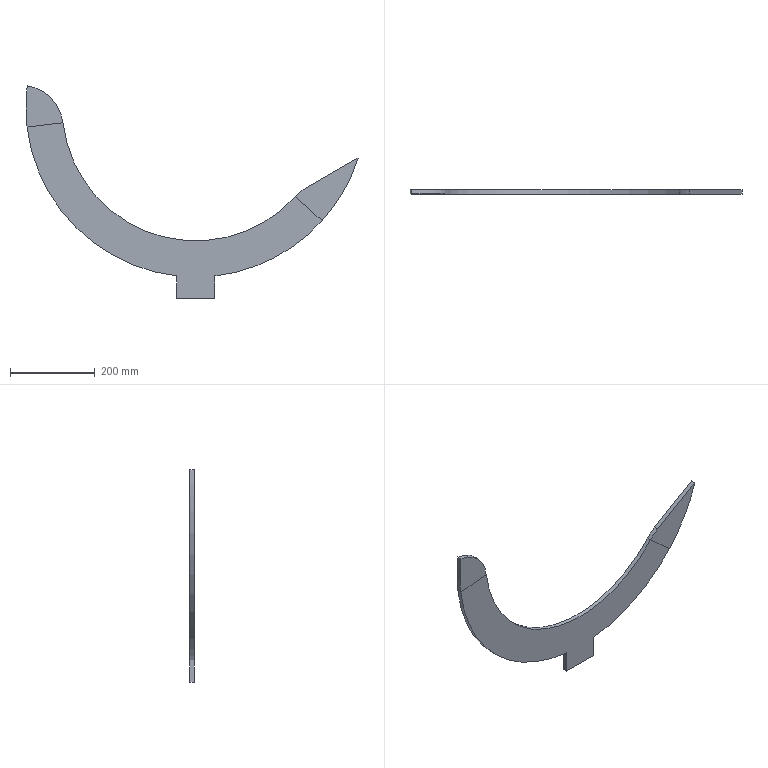Part | NX | features DATUM_CSYS 2, DIVIDE_FACE 1, EXTRUDE 1, SKETCH 1 | 1 solid | 15 faces | box 781.576 x 10 x 500 mm | volume 886213 mm3 | plane 10 | cylinder 5 | commonest cylinder face diameters 200 x2 800 x2 630 x1
STEP:
#1=CARTESIAN_POINT('',(-312.812,-5.,-37.063));
#2=VERTEX_POINT('',#1);
#3=CARTESIAN_POINT('',(234.054,-5.,-210.817));
#4=VERTEX_POINT('',#3);
#5=CARTESIAN_POINT('',(0.,-5.,0.));
#6=DIRECTION('',(0.,-1.,0.));
#7=DIRECTION('',(1.,0.,0.));
#8=AXIS2_PLACEMENT_3D('',#5,#6,#7);
#9=CIRCLE('',#8,315.);
#10=EDGE_CURVE('',#2,#4,#9,.T.);
#11=ORIENTED_EDGE('',*,*,#10,.F.);
#12=CARTESIAN_POINT('',(-397.221,-5.,-47.065));
#13=VERTEX_POINT('',#12);
#14=CARTESIAN_POINT('',(-312.812,-5.,-37.063));
#15=DIRECTION('',(-0.9931,0.,-0.1177));
#16=VECTOR('',#15,1000.);
#17=LINE('',#14,#16);
#18=EDGE_CURVE('',#2,#13,#17,.T.);
#19=ORIENTED_EDGE('',*,*,#18,.T.);
#20=CARTESIAN_POINT('',(-45.,-5.,-397.461));
#21=VERTEX_POINT('',#20);
#22=CARTESIAN_POINT('',(0.,-5.,0.));
#23=DIRECTION('',(0.,1.,0.));
#24=DIRECTION('',(1.,0.,0.));
#25=AXIS2_PLACEMENT_3D('',#22,#23,#24);
#26=CIRCLE('',#25,400.);
#27=EDGE_CURVE('',#21,#13,#26,.T.);
#28=ORIENTED_EDGE('',*,*,#27,.F.);
#29=CARTESIAN_POINT('',(-45.,-5.,-450.));
#30=VERTEX_POINT('',#29);
#31=CARTESIAN_POINT('',(-45.,-5.,-450.));
#32=DIRECTION('',(0.,0.,1.));
#33=VECTOR('',#32,1000.);
#34=LINE('',#31,#33);
#35=EDGE_CURVE('',#30,#21,#34,.T.);
#36=ORIENTED_EDGE('',*,*,#35,.F.);
#37=CARTESIAN_POINT('',(45.,-5.,-450.));
#38=VERTEX_POINT('',#37);
#39=CARTESIAN_POINT('',(45.,-5.,-450.));
#40=DIRECTION('',(-1.,0.,0.));
#41=VECTOR('',#40,1000.);
#42=LINE('',#39,#41);
#43=EDGE_CURVE('',#38,#30,#42,.T.);
#44=ORIENTED_EDGE('',*,*,#43,.F.);
#45=CARTESIAN_POINT('',(45.,-5.,-397.461));
#46=VERTEX_POINT('',#45);
#47=CARTESIAN_POINT('',(45.,-5.,-397.461));
#48=DIRECTION('',(0.,0.,-1.));
#49=VECTOR('',#48,1000.);
#50=LINE('',#47,#49);
#51=EDGE_CURVE('',#46,#38,#50,.T.);
#52=ORIENTED_EDGE('',*,*,#51,.F.);
#53=CARTESIAN_POINT('',(297.211,-5.,-267.704));
#54=VERTEX_POINT('',#53);
#55=CARTESIAN_POINT('',(0.,-5.,0.));
#56=DIRECTION('',(0.,1.,0.));
#57=DIRECTION('',(1.,0.,0.));
#58=AXIS2_PLACEMENT_3D('',#55,#56,#57);
#59=CIRCLE('',#58,400.);
#60=EDGE_CURVE('',#54,#46,#59,.T.);
#61=ORIENTED_EDGE('',*,*,#60,.F.);
#62=CARTESIAN_POINT('',(297.211,-5.,-267.704));
#63=DIRECTION('',(-0.743,0.,0.6693));
#64=VECTOR('',#63,1000.);
#65=LINE('',#62,#64);
#66=EDGE_CURVE('',#54,#4,#65,.T.);
#67=ORIENTED_EDGE('',*,*,#66,.T.);
#68=EDGE_LOOP('',(#11,#19,#28,#36,#44,#52,#61,#67));
#69=FACE_BOUND('',#68,.T.);
#70=CARTESIAN_POINT('',(0.,-5.,0.));
#71=DIRECTION('',(0.,-1.,0.));
#72=DIRECTION('',(0.,0.,-1.));
#73=AXIS2_PLACEMENT_3D('',#70,#71,#72);
#74=PLANE('',#73);
#75=ADVANCED_FACE('',(#69),#74,.T.);
#76=ORIENTED_EDGE('',*,*,#18,.F.);
#77=CARTESIAN_POINT('',(-396.863,-5.,50.));
#78=VERTEX_POINT('',#77);
#79=CARTESIAN_POINT('',(-412.117,-5.,-48.83));
#80=DIRECTION('',(0.,1.,0.));
#81=DIRECTION('',(1.,0.,0.));
#82=AXIS2_PLACEMENT_3D('',#79,#80,#81);
#83=CIRCLE('',#82,100.);
#84=EDGE_CURVE('',#78,#2,#83,.T.);
#85=ORIENTED_EDGE('',*,*,#84,.F.);
#86=CARTESIAN_POINT('',(0.,-5.,0.));
#87=DIRECTION('',(0.,1.,0.));
#88=DIRECTION('',(1.,0.,0.));
#89=AXIS2_PLACEMENT_3D('',#86,#87,#88);
#90=CIRCLE('',#89,400.);
#91=EDGE_CURVE('',#13,#78,#90,.T.);
#92=ORIENTED_EDGE('',*,*,#91,.F.);
#93=EDGE_LOOP('',(#76,#85,#92));
#94=FACE_BOUND('',#93,.T.);
#95=CARTESIAN_POINT('',(0.,-5.,0.));
#96=DIRECTION('',(0.,-1.,0.));
#97=DIRECTION('',(0.,0.,-1.));
#98=AXIS2_PLACEMENT_3D('',#95,#96,#97);
#99=PLANE('',#98);
#100=ADVANCED_FACE('',(#94),#99,.T.);
#101=CARTESIAN_POINT('',(-396.863,5.,50.));
#102=VERTEX_POINT('',#101);
#103=CARTESIAN_POINT('',(-312.812,5.,-37.063));
#104=VERTEX_POINT('',#103);
#105=CARTESIAN_POINT('',(-412.117,5.,-48.83));
#106=DIRECTION('',(0.,1.,0.));
#107=DIRECTION('',(1.,0.,0.));
#108=AXIS2_PLACEMENT_3D('',#105,#106,#107);
#109=CIRCLE('',#108,100.);
#110=EDGE_CURVE('',#102,#104,#109,.T.);
#111=ORIENTED_EDGE('',*,*,#110,.T.);
#112=CARTESIAN_POINT('',(-397.221,5.,-47.065));
#113=VERTEX_POINT('',#112);
#114=CARTESIAN_POINT('',(-312.812,5.,-37.063));
#115=DIRECTION('',(-0.9931,0.,-0.1177));
#116=VECTOR('',#115,1000.);
#117=LINE('',#114,#116);
#118=EDGE_CURVE('',#104,#113,#117,.T.);
#119=ORIENTED_EDGE('',*,*,#118,.T.);
#120=CARTESIAN_POINT('',(0.,5.,0.));
#121=DIRECTION('',(0.,1.,0.));
#122=DIRECTION('',(1.,0.,0.));
#123=AXIS2_PLACEMENT_3D('',#120,#121,#122);
#124=CIRCLE('',#123,400.);
#125=EDGE_CURVE('',#113,#102,#124,.T.);
#126=ORIENTED_EDGE('',*,*,#125,.T.);
#127=EDGE_LOOP('',(#111,#119,#126));
#128=FACE_BOUND('',#127,.T.);
#129=CARTESIAN_POINT('',(0.,5.,0.));
#130=DIRECTION('',(0.,-1.,0.));
#131=DIRECTION('',(0.,0.,-1.));
#132=AXIS2_PLACEMENT_3D('',#129,#130,#131);
#133=PLANE('',#132);
#134=ADVANCED_FACE('',(#128),#133,.F.);
#135=CARTESIAN_POINT('',(381.576,5.,-120.));
#136=VERTEX_POINT('',#135);
#137=CARTESIAN_POINT('',(297.211,5.,-267.704));
#138=VERTEX_POINT('',#137);
#139=CARTESIAN_POINT('',(0.,5.,0.));
#140=DIRECTION('',(0.,1.,0.));
#141=DIRECTION('',(1.,0.,0.));
#142=AXIS2_PLACEMENT_3D('',#139,#140,#141);
#143=CIRCLE('',#142,400.);
#144=EDGE_CURVE('',#136,#138,#143,.T.);
#145=ORIENTED_EDGE('',*,*,#144,.T.);
#146=CARTESIAN_POINT('',(234.054,5.,-210.817));
#147=VERTEX_POINT('',#146);
#148=CARTESIAN_POINT('',(297.211,5.,-267.704));
#149=DIRECTION('',(-0.743,0.,0.6693));
#150=VECTOR('',#149,1000.);
#151=LINE('',#148,#150);
#152=EDGE_CURVE('',#138,#147,#151,.T.);
#153=ORIENTED_EDGE('',*,*,#152,.T.);
#154=CARTESIAN_POINT('',(258.357,5.,-191.141));
#155=VERTEX_POINT('',#154);
#156=CARTESIAN_POINT('',(308.357,5.,-277.743));
#157=DIRECTION('',(0.,1.,0.));
#158=DIRECTION('',(1.,0.,0.));
#159=AXIS2_PLACEMENT_3D('',#156,#157,#158);
#160=CIRCLE('',#159,100.);
#161=EDGE_CURVE('',#147,#155,#160,.T.);
#162=ORIENTED_EDGE('',*,*,#161,.T.);
#163=CARTESIAN_POINT('',(258.357,5.,-191.141));
#164=DIRECTION('',(0.866,0.,0.5));
#165=VECTOR('',#164,1000.);
#166=LINE('',#163,#165);
#167=EDGE_CURVE('',#155,#136,#166,.T.);
#168=ORIENTED_EDGE('',*,*,#167,.T.);
#169=EDGE_LOOP('',(#145,#153,#162,#168));
#170=FACE_BOUND('',#169,.T.);
#171=CARTESIAN_POINT('',(0.,5.,0.));
#172=DIRECTION('',(0.,-1.,0.));
#173=DIRECTION('',(0.,0.,-1.));
#174=AXIS2_PLACEMENT_3D('',#171,#172,#173);
#175=PLANE('',#174);
#176=ADVANCED_FACE('',(#170),#175,.F.);
#177=CARTESIAN_POINT('',(0.,5.,0.));
#178=DIRECTION('',(0.,-1.,0.));
#179=DIRECTION('',(1.,0.,0.));
#180=AXIS2_PLACEMENT_3D('',#177,#178,#179);
#181=CIRCLE('',#180,315.);
#182=EDGE_CURVE('',#104,#147,#181,.T.);
#183=ORIENTED_EDGE('',*,*,#182,.F.);
#184=CARTESIAN_POINT('',(-312.812,-5.,-37.063));
#185=DIRECTION('',(0.,1.,0.));
#186=VECTOR('',#185,1000.);
#187=LINE('',#184,#186);
#188=EDGE_CURVE('',#2,#104,#187,.T.);
#189=ORIENTED_EDGE('',*,*,#188,.F.);
#190=ORIENTED_EDGE('',*,*,#10,.T.);
#191=CARTESIAN_POINT('',(234.054,-5.,-210.817));
#192=DIRECTION('',(0.,1.,0.));
#193=VECTOR('',#192,1000.);
#194=LINE('',#191,#193);
#195=EDGE_CURVE('',#4,#147,#194,.T.);
#196=ORIENTED_EDGE('',*,*,#195,.T.);
#197=EDGE_LOOP('',(#183,#189,#190,#196));
#198=FACE_BOUND('',#197,.T.);
#199=CARTESIAN_POINT('',(0.,-5.,0.));
#200=DIRECTION('',(0.,1.,0.));
#201=DIRECTION('',(0.,0.,1.));
#202=AXIS2_PLACEMENT_3D('',#199,#200,#201);
#203=CYLINDRICAL_SURFACE('',#202,315.);
#204=ADVANCED_FACE('',(#198),#203,.F.);
#205=ORIENTED_EDGE('',*,*,#161,.F.);
#206=ORIENTED_EDGE('',*,*,#195,.F.);
#207=CARTESIAN_POINT('',(258.357,-5.,-191.141));
#208=VERTEX_POINT('',#207);
#209=CARTESIAN_POINT('',(308.357,-5.,-277.743));
#210=DIRECTION('',(0.,1.,0.));
#211=DIRECTION('',(1.,0.,0.));
#212=AXIS2_PLACEMENT_3D('',#209,#210,#211);
#213=CIRCLE('',#212,100.);
#214=EDGE_CURVE('',#4,#208,#213,.T.);
#215=ORIENTED_EDGE('',*,*,#214,.T.);
#216=CARTESIAN_POINT('',(258.357,-5.,-191.141));
#217=DIRECTION('',(0.,1.,0.));
#218=VECTOR('',#217,1000.);
#219=LINE('',#216,#218);
#220=EDGE_CURVE('',#208,#155,#219,.T.);
#221=ORIENTED_EDGE('',*,*,#220,.T.);
#222=EDGE_LOOP('',(#205,#206,#215,#221));
#223=FACE_BOUND('',#222,.T.);
#224=CARTESIAN_POINT('',(308.357,-5.,-277.743));
#225=DIRECTION('',(0.,1.,0.));
#226=DIRECTION('',(0.,0.,1.));
#227=AXIS2_PLACEMENT_3D('',#224,#225,#226);
#228=CYLINDRICAL_SURFACE('',#227,100.);
#229=ADVANCED_FACE('',(#223),#228,.T.);
#230=ORIENTED_EDGE('',*,*,#167,.F.);
#231=ORIENTED_EDGE('',*,*,#220,.F.);
#232=CARTESIAN_POINT('',(381.576,-5.,-120.));
#233=VERTEX_POINT('',#232);
#234=CARTESIAN_POINT('',(258.357,-5.,-191.141));
#235=DIRECTION('',(0.866,0.,0.5));
#236=VECTOR('',#235,1000.);
#237=LINE('',#234,#236);
#238=EDGE_CURVE('',#208,#233,#237,.T.);
#239=ORIENTED_EDGE('',*,*,#238,.T.);
#240=CARTESIAN_POINT('',(381.576,-5.,-120.));
#241=DIRECTION('',(0.,1.,0.));
#242=VECTOR('',#241,1000.);
#243=LINE('',#240,#242);
#244=EDGE_CURVE('',#233,#136,#243,.T.);
#245=ORIENTED_EDGE('',*,*,#244,.T.);
#246=EDGE_LOOP('',(#230,#231,#239,#245));
#247=FACE_BOUND('',#246,.T.);
#248=CARTESIAN_POINT('',(258.357,-5.,-191.141));
#249=DIRECTION('',(-0.5,0.,0.866));
#250=DIRECTION('',(0.866,0.,0.5));
#251=AXIS2_PLACEMENT_3D('',#248,#249,#250);
#252=PLANE('',#251);
#253=ADVANCED_FACE('',(#247),#252,.T.);
#254=ORIENTED_EDGE('',*,*,#144,.F.);
#255=ORIENTED_EDGE('',*,*,#244,.F.);
#256=CARTESIAN_POINT('',(0.,-5.,0.));
#257=DIRECTION('',(0.,1.,0.));
#258=DIRECTION('',(1.,0.,0.));
#259=AXIS2_PLACEMENT_3D('',#256,#257,#258);
#260=CIRCLE('',#259,400.);
#261=EDGE_CURVE('',#233,#54,#260,.T.);
#262=ORIENTED_EDGE('',*,*,#261,.T.);
#263=ORIENTED_EDGE('',*,*,#60,.T.);
#264=CARTESIAN_POINT('',(45.,5.,-397.461));
#265=VERTEX_POINT('',#264);
#266=CARTESIAN_POINT('',(45.,-5.,-397.461));
#267=DIRECTION('',(0.,1.,0.));
#268=VECTOR('',#267,1000.);
#269=LINE('',#266,#268);
#270=EDGE_CURVE('',#46,#265,#269,.T.);
#271=ORIENTED_EDGE('',*,*,#270,.T.);
#272=CARTESIAN_POINT('',(0.,5.,0.));
#273=DIRECTION('',(0.,1.,0.));
#274=DIRECTION('',(1.,0.,0.));
#275=AXIS2_PLACEMENT_3D('',#272,#273,#274);
#276=CIRCLE('',#275,400.);
#277=EDGE_CURVE('',#138,#265,#276,.T.);
#278=ORIENTED_EDGE('',*,*,#277,.F.);
#279=EDGE_LOOP('',(#254,#255,#262,#263,#271,#278));
#280=FACE_BOUND('',#279,.T.);
#281=CARTESIAN_POINT('',(0.,-5.,0.));
#282=DIRECTION('',(0.,1.,0.));
#283=DIRECTION('',(0.,0.,1.));
#284=AXIS2_PLACEMENT_3D('',#281,#282,#283);
#285=CYLINDRICAL_SURFACE('',#284,400.);
#286=ADVANCED_FACE('',(#280),#285,.T.);
#287=CARTESIAN_POINT('',(45.,5.,-450.));
#288=VERTEX_POINT('',#287);
#289=CARTESIAN_POINT('',(45.,5.,-397.461));
#290=DIRECTION('',(0.,0.,-1.));
#291=VECTOR('',#290,1000.);
#292=LINE('',#289,#291);
#293=EDGE_CURVE('',#265,#288,#292,.T.);
#294=ORIENTED_EDGE('',*,*,#293,.F.);
#295=ORIENTED_EDGE('',*,*,#270,.F.);
#296=ORIENTED_EDGE('',*,*,#51,.T.);
#297=CARTESIAN_POINT('',(45.,-5.,-450.));
#298=DIRECTION('',(0.,1.,0.));
#299=VECTOR('',#298,1000.);
#300=LINE('',#297,#299);
#301=EDGE_CURVE('',#38,#288,#300,.T.);
#302=ORIENTED_EDGE('',*,*,#301,.T.);
#303=EDGE_LOOP('',(#294,#295,#296,#302));
#304=FACE_BOUND('',#303,.T.);
#305=CARTESIAN_POINT('',(45.,-5.,-397.461));
#306=DIRECTION('',(1.,0.,0.));
#307=DIRECTION('',(0.,0.,-1.));
#308=AXIS2_PLACEMENT_3D('',#305,#306,#307);
#309=PLANE('',#308);
#310=ADVANCED_FACE('',(#304),#309,.T.);
#311=CARTESIAN_POINT('',(-45.,5.,-450.));
#312=VERTEX_POINT('',#311);
#313=CARTESIAN_POINT('',(45.,5.,-450.));
#314=DIRECTION('',(-1.,0.,0.));
#315=VECTOR('',#314,1000.);
#316=LINE('',#313,#315);
#317=EDGE_CURVE('',#288,#312,#316,.T.);
#318=ORIENTED_EDGE('',*,*,#317,.F.);
#319=ORIENTED_EDGE('',*,*,#301,.F.);
#320=ORIENTED_EDGE('',*,*,#43,.T.);
#321=CARTESIAN_POINT('',(-45.,-5.,-450.));
#322=DIRECTION('',(0.,1.,0.));
#323=VECTOR('',#322,1000.);
#324=LINE('',#321,#323);
#325=EDGE_CURVE('',#30,#312,#324,.T.);
#326=ORIENTED_EDGE('',*,*,#325,.T.);
#327=EDGE_LOOP('',(#318,#319,#320,#326));
#328=FACE_BOUND('',#327,.T.);
#329=CARTESIAN_POINT('',(45.,-5.,-450.));
#330=DIRECTION('',(0.,0.,-1.));
#331=DIRECTION('',(-1.,0.,0.));
#332=AXIS2_PLACEMENT_3D('',#329,#330,#331);
#333=PLANE('',#332);
#334=ADVANCED_FACE('',(#328),#333,.T.);
#335=CARTESIAN_POINT('',(-45.,5.,-397.461));
#336=VERTEX_POINT('',#335);
#337=CARTESIAN_POINT('',(-45.,5.,-450.));
#338=DIRECTION('',(0.,0.,1.));
#339=VECTOR('',#338,1000.);
#340=LINE('',#337,#339);
#341=EDGE_CURVE('',#312,#336,#340,.T.);
#342=ORIENTED_EDGE('',*,*,#341,.F.);
#343=ORIENTED_EDGE('',*,*,#325,.F.);
#344=ORIENTED_EDGE('',*,*,#35,.T.);
#345=CARTESIAN_POINT('',(-45.,-5.,-397.461));
#346=DIRECTION('',(0.,1.,0.));
#347=VECTOR('',#346,1000.);
#348=LINE('',#345,#347);
#349=EDGE_CURVE('',#21,#336,#348,.T.);
#350=ORIENTED_EDGE('',*,*,#349,.T.);
#351=EDGE_LOOP('',(#342,#343,#344,#350));
#352=FACE_BOUND('',#351,.T.);
#353=CARTESIAN_POINT('',(-45.,-5.,-450.));
#354=DIRECTION('',(-1.,0.,0.));
#355=DIRECTION('',(0.,0.,1.));
#356=AXIS2_PLACEMENT_3D('',#353,#354,#355);
#357=PLANE('',#356);
#358=ADVANCED_FACE('',(#352),#357,.T.);
#359=CARTESIAN_POINT('',(0.,5.,0.));
#360=DIRECTION('',(0.,1.,0.));
#361=DIRECTION('',(1.,0.,0.));
#362=AXIS2_PLACEMENT_3D('',#359,#360,#361);
#363=CIRCLE('',#362,400.);
#364=EDGE_CURVE('',#336,#113,#363,.T.);
#365=ORIENTED_EDGE('',*,*,#364,.F.);
#366=ORIENTED_EDGE('',*,*,#349,.F.);
#367=ORIENTED_EDGE('',*,*,#27,.T.);
#368=ORIENTED_EDGE('',*,*,#91,.T.);
#369=CARTESIAN_POINT('',(-396.863,-5.,50.));
#370=DIRECTION('',(0.,1.,0.));
#371=VECTOR('',#370,1000.);
#372=LINE('',#369,#371);
#373=EDGE_CURVE('',#78,#102,#372,.T.);
#374=ORIENTED_EDGE('',*,*,#373,.T.);
#375=ORIENTED_EDGE('',*,*,#125,.F.);
#376=EDGE_LOOP('',(#365,#366,#367,#368,#374,#375));
#377=FACE_BOUND('',#376,.T.);
#378=CARTESIAN_POINT('',(0.,-5.,0.));
#379=DIRECTION('',(0.,1.,0.));
#380=DIRECTION('',(0.,0.,1.));
#381=AXIS2_PLACEMENT_3D('',#378,#379,#380);
#382=CYLINDRICAL_SURFACE('',#381,400.);
#383=ADVANCED_FACE('',(#377),#382,.T.);
#384=ORIENTED_EDGE('',*,*,#110,.F.);
#385=ORIENTED_EDGE('',*,*,#373,.F.);
#386=ORIENTED_EDGE('',*,*,#84,.T.);
#387=ORIENTED_EDGE('',*,*,#188,.T.);
#388=EDGE_LOOP('',(#384,#385,#386,#387));
#389=FACE_BOUND('',#388,.T.);
#390=CARTESIAN_POINT('',(-412.117,-5.,-48.83));
#391=DIRECTION('',(0.,1.,0.));
#392=DIRECTION('',(0.,0.,1.));
#393=AXIS2_PLACEMENT_3D('',#390,#391,#392);
#394=CYLINDRICAL_SURFACE('',#393,100.);
#395=ADVANCED_FACE('',(#389),#394,.T.);
#396=ORIENTED_EDGE('',*,*,#66,.F.);
#397=ORIENTED_EDGE('',*,*,#261,.F.);
#398=ORIENTED_EDGE('',*,*,#238,.F.);
#399=ORIENTED_EDGE('',*,*,#214,.F.);
#400=EDGE_LOOP('',(#396,#397,#398,#399));
#401=FACE_BOUND('',#400,.T.);
#402=CARTESIAN_POINT('',(0.,-5.,0.));
#403=DIRECTION('',(0.,-1.,0.));
#404=DIRECTION('',(0.,0.,-1.));
#405=AXIS2_PLACEMENT_3D('',#402,#403,#404);
#406=PLANE('',#405);
#407=ADVANCED_FACE('',(#401),#406,.T.);
#408=ORIENTED_EDGE('',*,*,#118,.F.);
#409=ORIENTED_EDGE('',*,*,#182,.T.);
#410=ORIENTED_EDGE('',*,*,#152,.F.);
#411=ORIENTED_EDGE('',*,*,#277,.T.);
#412=ORIENTED_EDGE('',*,*,#293,.T.);
#413=ORIENTED_EDGE('',*,*,#317,.T.);
#414=ORIENTED_EDGE('',*,*,#341,.T.);
#415=ORIENTED_EDGE('',*,*,#364,.T.);
#416=EDGE_LOOP('',(#408,#409,#410,#411,#412,#413,#414,#415));
#417=FACE_BOUND('',#416,.T.);
#418=CARTESIAN_POINT('',(0.,5.,0.));
#419=DIRECTION('',(0.,-1.,0.));
#420=DIRECTION('',(0.,0.,-1.));
#421=AXIS2_PLACEMENT_3D('',#418,#419,#420);
#422=PLANE('',#421);
#423=ADVANCED_FACE('',(#417),#422,.F.);
#424=CLOSED_SHELL('',(#75,#100,#134,#176,#204,#229,#253,#286,#310,#334,#358,#383,#395,#407,#423));
#425=MANIFOLD_SOLID_BREP('',#424);
#426=(LENGTH_UNIT()NAMED_UNIT(*)SI_UNIT(.MILLI.,.METRE.));
#427=UNCERTAINTY_MEASURE_WITH_UNIT(LENGTH_MEASURE(0.00001),#426,'','');
#428=(NAMED_UNIT(*)PLANE_ANGLE_UNIT()SI_UNIT($,.RADIAN.));
#429=(NAMED_UNIT(*)SI_UNIT($,.STERADIAN.)SOLID_ANGLE_UNIT());
#430=(GEOMETRIC_REPRESENTATION_CONTEXT(3)GLOBAL_UNCERTAINTY_ASSIGNED_CONTEXT((#427))GLOBAL_UNIT_ASSIGNED_CONTEXT((#426,#428,#429))REPRESENTATION_CONTEXT('',''));
#431=ADVANCED_BREP_SHAPE_REPRESENTATION('',(#425),#430);